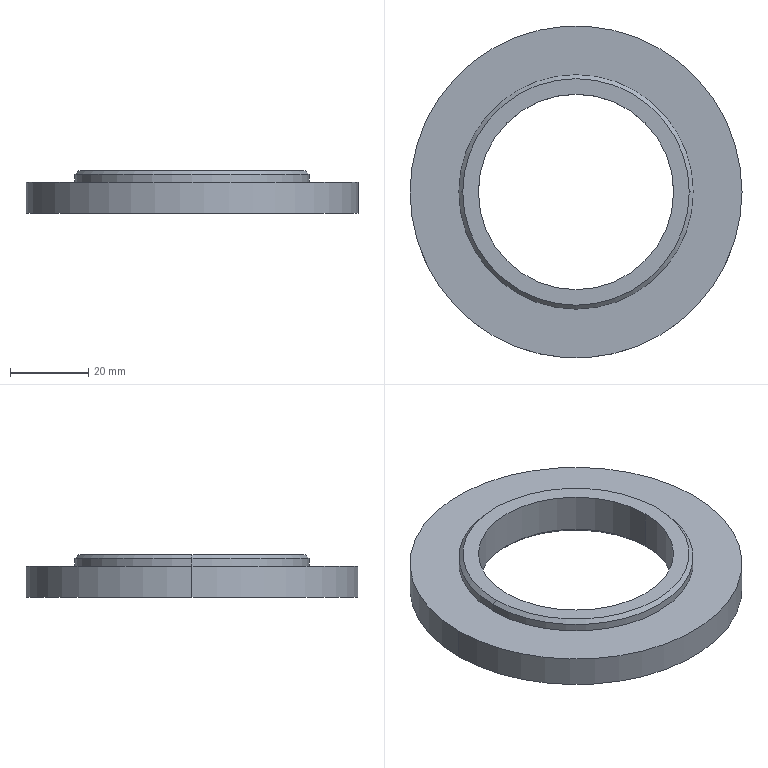Part | SolidWorks | features 3DProfileFeature 1, Chamfer 1, Extrusion 1, HoleWzd 1, ICE 1 | 1 solid | 37 faces | box 85 x 85 x 11 mm | volume 31782 mm3 | cylinder 18 | cone 16 | plane 3 | commonest cylinder face diameters 3.3 x12 50 x2 60 x2 85 x2
STEP:
#1=CARTESIAN_POINT('',(20.15,32.043,6.));
#2=VERTEX_POINT('',#1);
#3=CARTESIAN_POINT('',(16.85,32.043,6.));
#4=VERTEX_POINT('',#3);
#5=CARTESIAN_POINT('',(18.5,32.043,6.));
#6=DIRECTION('',(0.,0.,-1.));
#7=DIRECTION('',(-1.,0.,0.));
#8=AXIS2_PLACEMENT_3D('',#5,#6,#7);
#9=CIRCLE('',#8,1.65);
#10=EDGE_CURVE('',#2,#4,#9,.T.);
#11=ORIENTED_EDGE('',*,*,#10,.F.);
#12=CARTESIAN_POINT('',(20.15,32.043,0.));
#13=VERTEX_POINT('',#12);
#14=CARTESIAN_POINT('',(20.15,32.043,0.));
#15=DIRECTION('',(0.,0.,-1.));
#16=VECTOR('',#15,1000.);
#17=LINE('',#14,#16);
#18=EDGE_CURVE('',#2,#13,#17,.T.);
#19=ORIENTED_EDGE('',*,*,#18,.T.);
#20=CARTESIAN_POINT('',(16.85,32.043,0.));
#21=VERTEX_POINT('',#20);
#22=CARTESIAN_POINT('',(18.5,32.043,0.));
#23=DIRECTION('',(0.,0.,-1.));
#24=DIRECTION('',(-1.,0.,0.));
#25=AXIS2_PLACEMENT_3D('',#22,#23,#24);
#26=CIRCLE('',#25,1.65);
#27=EDGE_CURVE('',#13,#21,#26,.T.);
#28=ORIENTED_EDGE('',*,*,#27,.T.);
#29=CARTESIAN_POINT('',(16.85,32.043,0.));
#30=DIRECTION('',(0.,0.,-1.));
#31=VECTOR('',#30,1000.);
#32=LINE('',#29,#31);
#33=EDGE_CURVE('',#4,#21,#32,.T.);
#34=ORIENTED_EDGE('',*,*,#33,.F.);
#35=EDGE_LOOP('',(#11,#19,#28,#34));
#36=FACE_OUTER_BOUND('',#35,.T.);
#37=CARTESIAN_POINT('',(18.5,32.043,0.));
#38=DIRECTION('',(0.,0.,-1.));
#39=DIRECTION('',(-1.,0.,0.));
#40=AXIS2_PLACEMENT_3D('',#37,#38,#39);
#41=CYLINDRICAL_SURFACE('',#40,1.65);
#42=ADVANCED_FACE('',(#36),#41,.F.);
#43=CARTESIAN_POINT('',(18.5,32.043,6.991));
#44=VERTEX_POINT('',#43);
#45=CARTESIAN_POINT('',(16.85,32.043,6.));
#46=DIRECTION('',(-0.8572,0.,-0.515));
#47=VECTOR('',#46,1000.);
#48=LINE('',#45,#47);
#49=EDGE_CURVE('',#44,#4,#48,.T.);
#50=ORIENTED_EDGE('',*,*,#49,.F.);
#51=CARTESIAN_POINT('',(20.15,32.043,6.));
#52=DIRECTION('',(0.8572,0.,-0.515));
#53=VECTOR('',#52,1000.);
#54=LINE('',#51,#53);
#55=EDGE_CURVE('',#44,#2,#54,.T.);
#56=ORIENTED_EDGE('',*,*,#55,.T.);
#57=ORIENTED_EDGE('',*,*,#10,.T.);
#58=EDGE_LOOP('',(#50,#56,#57));
#59=FACE_OUTER_BOUND('',#58,.T.);
#60=CARTESIAN_POINT('',(18.5,32.043,6.));
#61=DIRECTION('',(0.,0.,-1.));
#62=DIRECTION('',(-1.,0.,0.));
#63=AXIS2_PLACEMENT_3D('',#60,#61,#62);
#64=CONICAL_SURFACE('',#63,1.65,1.03);
#65=ADVANCED_FACE('',(#59),#64,.F.);
#66=CARTESIAN_POINT('',(-16.85,32.043,6.));
#67=VERTEX_POINT('',#66);
#68=CARTESIAN_POINT('',(-20.15,32.043,6.));
#69=VERTEX_POINT('',#68);
#70=CARTESIAN_POINT('',(-18.5,32.043,6.));
#71=DIRECTION('',(0.,0.,-1.));
#72=DIRECTION('',(-1.,0.,0.));
#73=AXIS2_PLACEMENT_3D('',#70,#71,#72);
#74=CIRCLE('',#73,1.65);
#75=EDGE_CURVE('',#67,#69,#74,.T.);
#76=ORIENTED_EDGE('',*,*,#75,.F.);
#77=CARTESIAN_POINT('',(-16.85,32.043,0.));
#78=VERTEX_POINT('',#77);
#79=CARTESIAN_POINT('',(-16.85,32.043,0.));
#80=DIRECTION('',(0.,0.,-1.));
#81=VECTOR('',#80,1000.);
#82=LINE('',#79,#81);
#83=EDGE_CURVE('',#67,#78,#82,.T.);
#84=ORIENTED_EDGE('',*,*,#83,.T.);
#85=CARTESIAN_POINT('',(-20.15,32.043,0.));
#86=VERTEX_POINT('',#85);
#87=CARTESIAN_POINT('',(-18.5,32.043,0.));
#88=DIRECTION('',(0.,0.,-1.));
#89=DIRECTION('',(-1.,0.,0.));
#90=AXIS2_PLACEMENT_3D('',#87,#88,#89);
#91=CIRCLE('',#90,1.65);
#92=EDGE_CURVE('',#78,#86,#91,.T.);
#93=ORIENTED_EDGE('',*,*,#92,.T.);
#94=CARTESIAN_POINT('',(-20.15,32.043,0.));
#95=DIRECTION('',(0.,0.,-1.));
#96=VECTOR('',#95,1000.);
#97=LINE('',#94,#96);
#98=EDGE_CURVE('',#69,#86,#97,.T.);
#99=ORIENTED_EDGE('',*,*,#98,.F.);
#100=EDGE_LOOP('',(#76,#84,#93,#99));
#101=FACE_OUTER_BOUND('',#100,.T.);
#102=CARTESIAN_POINT('',(-18.5,32.043,0.));
#103=DIRECTION('',(0.,0.,-1.));
#104=DIRECTION('',(-1.,0.,0.));
#105=AXIS2_PLACEMENT_3D('',#102,#103,#104);
#106=CYLINDRICAL_SURFACE('',#105,1.65);
#107=ADVANCED_FACE('',(#101),#106,.F.);
#108=CARTESIAN_POINT('',(-18.5,32.043,6.991));
#109=VERTEX_POINT('',#108);
#110=CARTESIAN_POINT('',(-20.15,32.043,6.));
#111=DIRECTION('',(-0.8572,0.,-0.515));
#112=VECTOR('',#111,1000.);
#113=LINE('',#110,#112);
#114=EDGE_CURVE('',#109,#69,#113,.T.);
#115=ORIENTED_EDGE('',*,*,#114,.F.);
#116=CARTESIAN_POINT('',(-16.85,32.043,6.));
#117=DIRECTION('',(0.8572,0.,-0.515));
#118=VECTOR('',#117,1000.);
#119=LINE('',#116,#118);
#120=EDGE_CURVE('',#109,#67,#119,.T.);
#121=ORIENTED_EDGE('',*,*,#120,.T.);
#122=ORIENTED_EDGE('',*,*,#75,.T.);
#123=EDGE_LOOP('',(#115,#121,#122));
#124=FACE_OUTER_BOUND('',#123,.T.);
#125=CARTESIAN_POINT('',(-18.5,32.043,6.));
#126=DIRECTION('',(0.,0.,-1.));
#127=DIRECTION('',(-1.,0.,0.));
#128=AXIS2_PLACEMENT_3D('',#125,#126,#127);
#129=CONICAL_SURFACE('',#128,1.65,1.03);
#130=ADVANCED_FACE('',(#124),#129,.F.);
#131=CARTESIAN_POINT('',(-35.35,0.,6.));
#132=VERTEX_POINT('',#131);
#133=CARTESIAN_POINT('',(-38.65,0.,6.));
#134=VERTEX_POINT('',#133);
#135=CARTESIAN_POINT('',(-37.,0.,6.));
#136=DIRECTION('',(0.,0.,-1.));
#137=DIRECTION('',(-1.,0.,0.));
#138=AXIS2_PLACEMENT_3D('',#135,#136,#137);
#139=CIRCLE('',#138,1.65);
#140=EDGE_CURVE('',#132,#134,#139,.T.);
#141=ORIENTED_EDGE('',*,*,#140,.F.);
#142=CARTESIAN_POINT('',(-35.35,0.,0.));
#143=VERTEX_POINT('',#142);
#144=CARTESIAN_POINT('',(-35.35,0.,0.));
#145=DIRECTION('',(0.,0.,-1.));
#146=VECTOR('',#145,1000.);
#147=LINE('',#144,#146);
#148=EDGE_CURVE('',#132,#143,#147,.T.);
#149=ORIENTED_EDGE('',*,*,#148,.T.);
#150=CARTESIAN_POINT('',(-38.65,0.,0.));
#151=VERTEX_POINT('',#150);
#152=CARTESIAN_POINT('',(-37.,0.,0.));
#153=DIRECTION('',(0.,0.,-1.));
#154=DIRECTION('',(-1.,0.,0.));
#155=AXIS2_PLACEMENT_3D('',#152,#153,#154);
#156=CIRCLE('',#155,1.65);
#157=EDGE_CURVE('',#143,#151,#156,.T.);
#158=ORIENTED_EDGE('',*,*,#157,.T.);
#159=CARTESIAN_POINT('',(-38.65,0.,0.));
#160=DIRECTION('',(0.,0.,-1.));
#161=VECTOR('',#160,1000.);
#162=LINE('',#159,#161);
#163=EDGE_CURVE('',#134,#151,#162,.T.);
#164=ORIENTED_EDGE('',*,*,#163,.F.);
#165=EDGE_LOOP('',(#141,#149,#158,#164));
#166=FACE_OUTER_BOUND('',#165,.T.);
#167=CARTESIAN_POINT('',(-37.,0.,0.));
#168=DIRECTION('',(0.,0.,-1.));
#169=DIRECTION('',(-1.,0.,0.));
#170=AXIS2_PLACEMENT_3D('',#167,#168,#169);
#171=CYLINDRICAL_SURFACE('',#170,1.65);
#172=ADVANCED_FACE('',(#166),#171,.F.);
#173=CARTESIAN_POINT('',(-37.,0.,6.991));
#174=VERTEX_POINT('',#173);
#175=CARTESIAN_POINT('',(-38.65,0.,6.));
#176=DIRECTION('',(-0.8572,0.,-0.515));
#177=VECTOR('',#176,1000.);
#178=LINE('',#175,#177);
#179=EDGE_CURVE('',#174,#134,#178,.T.);
#180=ORIENTED_EDGE('',*,*,#179,.F.);
#181=CARTESIAN_POINT('',(-35.35,0.,6.));
#182=DIRECTION('',(0.8572,0.,-0.515));
#183=VECTOR('',#182,1000.);
#184=LINE('',#181,#183);
#185=EDGE_CURVE('',#174,#132,#184,.T.);
#186=ORIENTED_EDGE('',*,*,#185,.T.);
#187=ORIENTED_EDGE('',*,*,#140,.T.);
#188=EDGE_LOOP('',(#180,#186,#187));
#189=FACE_OUTER_BOUND('',#188,.T.);
#190=CARTESIAN_POINT('',(-37.,0.,6.));
#191=DIRECTION('',(0.,0.,-1.));
#192=DIRECTION('',(-1.,0.,0.));
#193=AXIS2_PLACEMENT_3D('',#190,#191,#192);
#194=CONICAL_SURFACE('',#193,1.65,1.03);
#195=ADVANCED_FACE('',(#189),#194,.F.);
#196=CARTESIAN_POINT('',(-16.85,-32.043,6.));
#197=VERTEX_POINT('',#196);
#198=CARTESIAN_POINT('',(-20.15,-32.043,6.));
#199=VERTEX_POINT('',#198);
#200=CARTESIAN_POINT('',(-18.5,-32.043,6.));
#201=DIRECTION('',(0.,0.,-1.));
#202=DIRECTION('',(-1.,0.,0.));
#203=AXIS2_PLACEMENT_3D('',#200,#201,#202);
#204=CIRCLE('',#203,1.65);
#205=EDGE_CURVE('',#197,#199,#204,.T.);
#206=ORIENTED_EDGE('',*,*,#205,.F.);
#207=CARTESIAN_POINT('',(-16.85,-32.043,0.));
#208=VERTEX_POINT('',#207);
#209=CARTESIAN_POINT('',(-16.85,-32.043,0.));
#210=DIRECTION('',(0.,0.,-1.));
#211=VECTOR('',#210,1000.);
#212=LINE('',#209,#211);
#213=EDGE_CURVE('',#197,#208,#212,.T.);
#214=ORIENTED_EDGE('',*,*,#213,.T.);
#215=CARTESIAN_POINT('',(-20.15,-32.043,0.));
#216=VERTEX_POINT('',#215);
#217=CARTESIAN_POINT('',(-18.5,-32.043,0.));
#218=DIRECTION('',(0.,0.,-1.));
#219=DIRECTION('',(-1.,0.,0.));
#220=AXIS2_PLACEMENT_3D('',#217,#218,#219);
#221=CIRCLE('',#220,1.65);
#222=EDGE_CURVE('',#208,#216,#221,.T.);
#223=ORIENTED_EDGE('',*,*,#222,.T.);
#224=CARTESIAN_POINT('',(-20.15,-32.043,0.));
#225=DIRECTION('',(0.,0.,-1.));
#226=VECTOR('',#225,1000.);
#227=LINE('',#224,#226);
#228=EDGE_CURVE('',#199,#216,#227,.T.);
#229=ORIENTED_EDGE('',*,*,#228,.F.);
#230=EDGE_LOOP('',(#206,#214,#223,#229));
#231=FACE_OUTER_BOUND('',#230,.T.);
#232=CARTESIAN_POINT('',(-18.5,-32.043,0.));
#233=DIRECTION('',(0.,0.,-1.));
#234=DIRECTION('',(-1.,0.,0.));
#235=AXIS2_PLACEMENT_3D('',#232,#233,#234);
#236=CYLINDRICAL_SURFACE('',#235,1.65);
#237=ADVANCED_FACE('',(#231),#236,.F.);
#238=CARTESIAN_POINT('',(-18.5,-32.043,6.991));
#239=VERTEX_POINT('',#238);
#240=CARTESIAN_POINT('',(-20.15,-32.043,6.));
#241=DIRECTION('',(-0.8572,0.,-0.515));
#242=VECTOR('',#241,1000.);
#243=LINE('',#240,#242);
#244=EDGE_CURVE('',#239,#199,#243,.T.);
#245=ORIENTED_EDGE('',*,*,#244,.F.);
#246=CARTESIAN_POINT('',(-16.85,-32.043,6.));
#247=DIRECTION('',(0.8572,0.,-0.515));
#248=VECTOR('',#247,1000.);
#249=LINE('',#246,#248);
#250=EDGE_CURVE('',#239,#197,#249,.T.);
#251=ORIENTED_EDGE('',*,*,#250,.T.);
#252=ORIENTED_EDGE('',*,*,#205,.T.);
#253=EDGE_LOOP('',(#245,#251,#252));
#254=FACE_OUTER_BOUND('',#253,.T.);
#255=CARTESIAN_POINT('',(-18.5,-32.043,6.));
#256=DIRECTION('',(0.,0.,-1.));
#257=DIRECTION('',(-1.,0.,0.));
#258=AXIS2_PLACEMENT_3D('',#255,#256,#257);
#259=CONICAL_SURFACE('',#258,1.65,1.03);
#260=ADVANCED_FACE('',(#254),#259,.F.);
#261=CARTESIAN_POINT('',(20.15,-32.043,6.));
#262=VERTEX_POINT('',#261);
#263=CARTESIAN_POINT('',(16.85,-32.043,6.));
#264=VERTEX_POINT('',#263);
#265=CARTESIAN_POINT('',(18.5,-32.043,6.));
#266=DIRECTION('',(0.,0.,-1.));
#267=DIRECTION('',(-1.,0.,0.));
#268=AXIS2_PLACEMENT_3D('',#265,#266,#267);
#269=CIRCLE('',#268,1.65);
#270=EDGE_CURVE('',#262,#264,#269,.T.);
#271=ORIENTED_EDGE('',*,*,#270,.F.);
#272=CARTESIAN_POINT('',(20.15,-32.043,0.));
#273=VERTEX_POINT('',#272);
#274=CARTESIAN_POINT('',(20.15,-32.043,0.));
#275=DIRECTION('',(0.,0.,-1.));
#276=VECTOR('',#275,1000.);
#277=LINE('',#274,#276);
#278=EDGE_CURVE('',#262,#273,#277,.T.);
#279=ORIENTED_EDGE('',*,*,#278,.T.);
#280=CARTESIAN_POINT('',(16.85,-32.043,0.));
#281=VERTEX_POINT('',#280);
#282=CARTESIAN_POINT('',(18.5,-32.043,0.));
#283=DIRECTION('',(0.,0.,-1.));
#284=DIRECTION('',(-1.,0.,0.));
#285=AXIS2_PLACEMENT_3D('',#282,#283,#284);
#286=CIRCLE('',#285,1.65);
#287=EDGE_CURVE('',#273,#281,#286,.T.);
#288=ORIENTED_EDGE('',*,*,#287,.T.);
#289=CARTESIAN_POINT('',(16.85,-32.043,0.));
#290=DIRECTION('',(0.,0.,-1.));
#291=VECTOR('',#290,1000.);
#292=LINE('',#289,#291);
#293=EDGE_CURVE('',#264,#281,#292,.T.);
#294=ORIENTED_EDGE('',*,*,#293,.F.);
#295=EDGE_LOOP('',(#271,#279,#288,#294));
#296=FACE_OUTER_BOUND('',#295,.T.);
#297=CARTESIAN_POINT('',(18.5,-32.043,0.));
#298=DIRECTION('',(0.,0.,-1.));
#299=DIRECTION('',(-1.,0.,0.));
#300=AXIS2_PLACEMENT_3D('',#297,#298,#299);
#301=CYLINDRICAL_SURFACE('',#300,1.65);
#302=ADVANCED_FACE('',(#296),#301,.F.);
#303=CARTESIAN_POINT('',(18.5,-32.043,6.991));
#304=VERTEX_POINT('',#303);
#305=CARTESIAN_POINT('',(16.85,-32.043,6.));
#306=DIRECTION('',(-0.8572,0.,-0.515));
#307=VECTOR('',#306,1000.);
#308=LINE('',#305,#307);
#309=EDGE_CURVE('',#304,#264,#308,.T.);
#310=ORIENTED_EDGE('',*,*,#309,.F.);
#311=CARTESIAN_POINT('',(20.15,-32.043,6.));
#312=DIRECTION('',(0.8572,0.,-0.515));
#313=VECTOR('',#312,1000.);
#314=LINE('',#311,#313);
#315=EDGE_CURVE('',#304,#262,#314,.T.);
#316=ORIENTED_EDGE('',*,*,#315,.T.);
#317=ORIENTED_EDGE('',*,*,#270,.T.);
#318=EDGE_LOOP('',(#310,#316,#317));
#319=FACE_OUTER_BOUND('',#318,.T.);
#320=CARTESIAN_POINT('',(18.5,-32.043,6.));
#321=DIRECTION('',(0.,0.,-1.));
#322=DIRECTION('',(-1.,0.,0.));
#323=AXIS2_PLACEMENT_3D('',#320,#321,#322);
#324=CONICAL_SURFACE('',#323,1.65,1.03);
#325=ADVANCED_FACE('',(#319),#324,.F.);
#326=CARTESIAN_POINT('',(38.65,0.,6.));
#327=VERTEX_POINT('',#326);
#328=CARTESIAN_POINT('',(35.35,0.,6.));
#329=VERTEX_POINT('',#328);
#330=CARTESIAN_POINT('',(37.,0.,6.));
#331=DIRECTION('',(0.,0.,-1.));
#332=DIRECTION('',(-1.,0.,0.));
#333=AXIS2_PLACEMENT_3D('',#330,#331,#332);
#334=CIRCLE('',#333,1.65);
#335=EDGE_CURVE('',#327,#329,#334,.T.);
#336=ORIENTED_EDGE('',*,*,#335,.F.);
#337=CARTESIAN_POINT('',(38.65,0.,0.));
#338=VERTEX_POINT('',#337);
#339=CARTESIAN_POINT('',(38.65,0.,0.));
#340=DIRECTION('',(0.,0.,-1.));
#341=VECTOR('',#340,1000.);
#342=LINE('',#339,#341);
#343=EDGE_CURVE('',#327,#338,#342,.T.);
#344=ORIENTED_EDGE('',*,*,#343,.T.);
#345=CARTESIAN_POINT('',(35.35,0.,0.));
#346=VERTEX_POINT('',#345);
#347=CARTESIAN_POINT('',(37.,0.,0.));
#348=DIRECTION('',(0.,0.,-1.));
#349=DIRECTION('',(-1.,0.,0.));
#350=AXIS2_PLACEMENT_3D('',#347,#348,#349);
#351=CIRCLE('',#350,1.65);
#352=EDGE_CURVE('',#338,#346,#351,.T.);
#353=ORIENTED_EDGE('',*,*,#352,.T.);
#354=CARTESIAN_POINT('',(35.35,0.,0.));
#355=DIRECTION('',(0.,0.,-1.));
#356=VECTOR('',#355,1000.);
#357=LINE('',#354,#356);
#358=EDGE_CURVE('',#329,#346,#357,.T.);
#359=ORIENTED_EDGE('',*,*,#358,.F.);
#360=EDGE_LOOP('',(#336,#344,#353,#359));
#361=FACE_OUTER_BOUND('',#360,.T.);
#362=CARTESIAN_POINT('',(37.,0.,0.));
#363=DIRECTION('',(0.,0.,-1.));
#364=DIRECTION('',(-1.,0.,0.));
#365=AXIS2_PLACEMENT_3D('',#362,#363,#364);
#366=CYLINDRICAL_SURFACE('',#365,1.65);
#367=ADVANCED_FACE('',(#361),#366,.F.);
#368=CARTESIAN_POINT('',(37.,0.,6.991));
#369=VERTEX_POINT('',#368);
#370=CARTESIAN_POINT('',(35.35,0.,6.));
#371=DIRECTION('',(-0.8572,0.,-0.515));
#372=VECTOR('',#371,1000.);
#373=LINE('',#370,#372);
#374=EDGE_CURVE('',#369,#329,#373,.T.);
#375=ORIENTED_EDGE('',*,*,#374,.F.);
#376=CARTESIAN_POINT('',(38.65,0.,6.));
#377=DIRECTION('',(0.8572,0.,-0.515));
#378=VECTOR('',#377,1000.);
#379=LINE('',#376,#378);
#380=EDGE_CURVE('',#369,#327,#379,.T.);
#381=ORIENTED_EDGE('',*,*,#380,.T.);
#382=ORIENTED_EDGE('',*,*,#335,.T.);
#383=EDGE_LOOP('',(#375,#381,#382));
#384=FACE_OUTER_BOUND('',#383,.T.);
#385=CARTESIAN_POINT('',(37.,0.,6.));
#386=DIRECTION('',(0.,0.,-1.));
#387=DIRECTION('',(-1.,0.,0.));
#388=AXIS2_PLACEMENT_3D('',#385,#386,#387);
#389=CONICAL_SURFACE('',#388,1.65,1.03);
#390=ADVANCED_FACE('',(#384),#389,.F.);
#391=CARTESIAN_POINT('',(25.,0.,1.));
#392=VERTEX_POINT('',#391);
#393=CARTESIAN_POINT('',(-25.,0.,1.));
#394=VERTEX_POINT('',#393);
#395=CARTESIAN_POINT('',(0.,0.,1.));
#396=DIRECTION('',(0.,0.,-1.));
#397=DIRECTION('',(1.,0.,0.));
#398=AXIS2_PLACEMENT_3D('',#395,#396,#397);
#399=CIRCLE('',#398,25.);
#400=EDGE_CURVE('',#392,#394,#399,.T.);
#401=ORIENTED_EDGE('',*,*,#400,.F.);
#402=CARTESIAN_POINT('',(26.,0.,0.));
#403=VERTEX_POINT('',#402);
#404=CARTESIAN_POINT('',(26.,0.,0.));
#405=DIRECTION('',(0.7071,0.,-0.7071));
#406=VECTOR('',#405,1000.);
#407=LINE('',#404,#406);
#408=EDGE_CURVE('',#392,#403,#407,.T.);
#409=ORIENTED_EDGE('',*,*,#408,.T.);
#410=CARTESIAN_POINT('',(-26.,0.,0.));
#411=VERTEX_POINT('',#410);
#412=CARTESIAN_POINT('',(0.,0.,0.));
#413=DIRECTION('',(0.,0.,1.));
#414=DIRECTION('',(1.,0.,0.));
#415=AXIS2_PLACEMENT_3D('',#412,#413,#414);
#416=CIRCLE('',#415,26.);
#417=EDGE_CURVE('',#411,#403,#416,.T.);
#418=ORIENTED_EDGE('',*,*,#417,.F.);
#419=CARTESIAN_POINT('',(-26.,0.,0.));
#420=DIRECTION('',(-0.7071,0.,-0.7071));
#421=VECTOR('',#420,1000.);
#422=LINE('',#419,#421);
#423=EDGE_CURVE('',#394,#411,#422,.T.);
#424=ORIENTED_EDGE('',*,*,#423,.F.);
#425=EDGE_LOOP('',(#401,#409,#418,#424));
#426=FACE_OUTER_BOUND('',#425,.T.);
#427=CARTESIAN_POINT('',(0.,0.,0.));
#428=DIRECTION('',(0.,0.,-1.));
#429=DIRECTION('',(-1.,0.,0.));
#430=AXIS2_PLACEMENT_3D('',#427,#428,#429);
#431=CONICAL_SURFACE('',#430,26.,0.7854);
#432=ADVANCED_FACE('',(#426),#431,.F.);
#433=CARTESIAN_POINT('',(29.,0.,11.));
#434=VERTEX_POINT('',#433);
#435=CARTESIAN_POINT('',(-29.,0.,11.));
#436=VERTEX_POINT('',#435);
#437=CARTESIAN_POINT('',(0.,0.,11.));
#438=DIRECTION('',(0.,0.,1.));
#439=DIRECTION('',(1.,0.,0.));
#440=AXIS2_PLACEMENT_3D('',#437,#438,#439);
#441=CIRCLE('',#440,29.);
#442=EDGE_CURVE('',#434,#436,#441,.T.);
#443=ORIENTED_EDGE('',*,*,#442,.F.);
#444=CARTESIAN_POINT('',(30.,0.,10.));
#445=VERTEX_POINT('',#444);
#446=CARTESIAN_POINT('',(29.,0.,11.));
#447=DIRECTION('',(0.7071,0.,-0.7071));
#448=VECTOR('',#447,1000.);
#449=LINE('',#446,#448);
#450=EDGE_CURVE('',#434,#445,#449,.T.);
#451=ORIENTED_EDGE('',*,*,#450,.T.);
#452=CARTESIAN_POINT('',(-30.,0.,10.));
#453=VERTEX_POINT('',#452);
#454=CARTESIAN_POINT('',(0.,0.,10.));
#455=DIRECTION('',(0.,0.,-1.));
#456=DIRECTION('',(1.,0.,0.));
#457=AXIS2_PLACEMENT_3D('',#454,#455,#456);
#458=CIRCLE('',#457,30.);
#459=EDGE_CURVE('',#453,#445,#458,.T.);
#460=ORIENTED_EDGE('',*,*,#459,.F.);
#461=CARTESIAN_POINT('',(-29.,0.,11.));
#462=DIRECTION('',(-0.7071,0.,-0.7071));
#463=VECTOR('',#462,1000.);
#464=LINE('',#461,#463);
#465=EDGE_CURVE('',#436,#453,#464,.T.);
#466=ORIENTED_EDGE('',*,*,#465,.F.);
#467=EDGE_LOOP('',(#443,#451,#460,#466));
#468=FACE_OUTER_BOUND('',#467,.T.);
#469=CARTESIAN_POINT('',(0.,0.,11.));
#470=DIRECTION('',(0.,0.,-1.));
#471=DIRECTION('',(-1.,0.,0.));
#472=AXIS2_PLACEMENT_3D('',#469,#470,#471);
#473=CONICAL_SURFACE('',#472,29.,0.7854);
#474=ADVANCED_FACE('',(#468),#473,.T.);
#475=ORIENTED_EDGE('',*,*,#459,.T.);
#476=CARTESIAN_POINT('',(30.,0.,8.));
#477=VERTEX_POINT('',#476);
#478=CARTESIAN_POINT('',(30.,0.,11.));
#479=DIRECTION('',(0.,0.,-1.));
#480=VECTOR('',#479,1000.);
#481=LINE('',#478,#480);
#482=EDGE_CURVE('',#445,#477,#481,.T.);
#483=ORIENTED_EDGE('',*,*,#482,.T.);
#484=CARTESIAN_POINT('',(-30.,0.,8.));
#485=VERTEX_POINT('',#484);
#486=CARTESIAN_POINT('',(0.,0.,8.));
#487=DIRECTION('',(0.,0.,1.));
#488=DIRECTION('',(1.,0.,0.));
#489=AXIS2_PLACEMENT_3D('',#486,#487,#488);
#490=CIRCLE('',#489,30.);
#491=EDGE_CURVE('',#477,#485,#490,.T.);
#492=ORIENTED_EDGE('',*,*,#491,.T.);
#493=CARTESIAN_POINT('',(-30.,0.,11.));
#494=DIRECTION('',(0.,0.,-1.));
#495=VECTOR('',#494,1000.);
#496=LINE('',#493,#495);
#497=EDGE_CURVE('',#453,#485,#496,.T.);
#498=ORIENTED_EDGE('',*,*,#497,.F.);
#499=EDGE_LOOP('',(#475,#483,#492,#498));
#500=FACE_OUTER_BOUND('',#499,.T.);
#501=CARTESIAN_POINT('',(0.,0.,11.));
#502=DIRECTION('',(0.,0.,-1.));
#503=DIRECTION('',(-1.,0.,0.));
#504=AXIS2_PLACEMENT_3D('',#501,#502,#503);
#505=CYLINDRICAL_SURFACE('',#504,30.);
#506=ADVANCED_FACE('',(#500),#505,.T.);
#507=CARTESIAN_POINT('',(-25.,0.,11.));
#508=VERTEX_POINT('',#507);
#509=CARTESIAN_POINT('',(25.,0.,11.));
#510=VERTEX_POINT('',#509);
#511=CARTESIAN_POINT('',(0.,0.,11.));
#512=DIRECTION('',(0.,0.,1.));
#513=DIRECTION('',(1.,0.,0.));
#514=AXIS2_PLACEMENT_3D('',#511,#512,#513);
#515=CIRCLE('',#514,25.);
#516=EDGE_CURVE('',#508,#510,#515,.T.);
#517=ORIENTED_EDGE('',*,*,#516,.T.);
#518=CARTESIAN_POINT('',(25.,0.,8.));
#519=DIRECTION('',(0.,0.,-1.));
#520=VECTOR('',#519,1000.);
#521=LINE('',#518,#520);
#522=EDGE_CURVE('',#510,#392,#521,.T.);
#523=ORIENTED_EDGE('',*,*,#522,.T.);
#524=ORIENTED_EDGE('',*,*,#400,.T.);
#525=CARTESIAN_POINT('',(-25.,0.,8.));
#526=DIRECTION('',(0.,0.,-1.));
#527=VECTOR('',#526,1000.);
#528=LINE('',#525,#527);
#529=EDGE_CURVE('',#508,#394,#528,.T.);
#530=ORIENTED_EDGE('',*,*,#529,.F.);
#531=EDGE_LOOP('',(#517,#523,#524,#530));
#532=FACE_OUTER_BOUND('',#531,.T.);
#533=CARTESIAN_POINT('',(0.,0.,8.));
#534=DIRECTION('',(0.,0.,-1.));
#535=DIRECTION('',(-1.,0.,0.));
#536=AXIS2_PLACEMENT_3D('',#533,#534,#535);
#537=CYLINDRICAL_SURFACE('',#536,25.);
#538=ADVANCED_FACE('',(#532),#537,.F.);
#539=CARTESIAN_POINT('',(42.5,0.,8.));
#540=VERTEX_POINT('',#539);
#541=CARTESIAN_POINT('',(-42.5,0.,8.));
#542=VERTEX_POINT('',#541);
#543=CARTESIAN_POINT('',(0.,0.,8.));
#544=DIRECTION('',(0.,0.,1.));
#545=DIRECTION('',(1.,0.,0.));
#546=AXIS2_PLACEMENT_3D('',#543,#544,#545);
#547=CIRCLE('',#546,42.5);
#548=EDGE_CURVE('',#540,#542,#547,.T.);
#549=ORIENTED_EDGE('',*,*,#548,.F.);
#550=CARTESIAN_POINT('',(42.5,0.,0.));
#551=VERTEX_POINT('',#550);
#552=CARTESIAN_POINT('',(42.5,0.,8.));
#553=DIRECTION('',(0.,0.,-1.));
#554=VECTOR('',#553,1000.);
#555=LINE('',#552,#554);
#556=EDGE_CURVE('',#540,#551,#555,.T.);
#557=ORIENTED_EDGE('',*,*,#556,.T.);
#558=CARTESIAN_POINT('',(-42.5,0.,0.));
#559=VERTEX_POINT('',#558);
#560=CARTESIAN_POINT('',(0.,0.,0.));
#561=DIRECTION('',(0.,0.,1.));
#562=DIRECTION('',(1.,0.,0.));
#563=AXIS2_PLACEMENT_3D('',#560,#561,#562);
#564=CIRCLE('',#563,42.5);
#565=EDGE_CURVE('',#551,#559,#564,.T.);
#566=ORIENTED_EDGE('',*,*,#565,.T.);
#567=CARTESIAN_POINT('',(-42.5,0.,8.));
#568=DIRECTION('',(0.,0.,-1.));
#569=VECTOR('',#568,1000.);
#570=LINE('',#567,#569);
#571=EDGE_CURVE('',#542,#559,#570,.T.);
#572=ORIENTED_EDGE('',*,*,#571,.F.);
#573=EDGE_LOOP('',(#549,#557,#566,#572));
#574=FACE_OUTER_BOUND('',#573,.T.);
#575=CARTESIAN_POINT('',(0.,0.,8.));
#576=DIRECTION('',(0.,0.,-1.));
#577=DIRECTION('',(-1.,0.,0.));
#578=AXIS2_PLACEMENT_3D('',#575,#576,#577);
#579=CYLINDRICAL_SURFACE('',#578,42.5);
#580=ADVANCED_FACE('',(#574),#579,.T.);
#581=CARTESIAN_POINT('',(0.,0.,8.));
#582=DIRECTION('',(0.,0.,1.));
#583=DIRECTION('',(1.,0.,0.));
#584=AXIS2_PLACEMENT_3D('',#581,#582,#583);
#585=CIRCLE('',#584,42.5);
#586=EDGE_CURVE('',#542,#540,#585,.T.);
#587=ORIENTED_EDGE('',*,*,#586,.T.);
#588=ORIENTED_EDGE('',*,*,#548,.T.);
#589=EDGE_LOOP('',(#587,#588));
#590=FACE_OUTER_BOUND('',#589,.T.);
#591=CARTESIAN_POINT('',(0.,0.,8.));
#592=DIRECTION('',(0.,0.,1.));
#593=DIRECTION('',(1.,0.,0.));
#594=AXIS2_PLACEMENT_3D('',#591,#592,#593);
#595=CIRCLE('',#594,30.);
#596=EDGE_CURVE('',#485,#477,#595,.T.);
#597=ORIENTED_EDGE('',*,*,#596,.F.);
#598=ORIENTED_EDGE('',*,*,#491,.F.);
#599=EDGE_LOOP('',(#597,#598));
#600=FACE_BOUND('',#599,.T.);
#601=CARTESIAN_POINT('',(0.,0.,8.));
#602=DIRECTION('',(0.,0.,1.));
#603=DIRECTION('',(1.,0.,0.));
#604=AXIS2_PLACEMENT_3D('',#601,#602,#603);
#605=PLANE('',#604);
#606=ADVANCED_FACE('',(#590,#600),#605,.T.);
#607=CARTESIAN_POINT('',(18.5,32.043,0.));
#608=DIRECTION('',(0.,0.,-1.));
#609=DIRECTION('',(-1.,0.,0.));
#610=AXIS2_PLACEMENT_3D('',#607,#608,#609);
#611=CIRCLE('',#610,1.65);
#612=EDGE_CURVE('',#21,#13,#611,.T.);
#613=ORIENTED_EDGE('',*,*,#612,.F.);
#614=ORIENTED_EDGE('',*,*,#27,.F.);
#615=EDGE_LOOP('',(#613,#614));
#616=FACE_BOUND('',#615,.T.);
#617=CARTESIAN_POINT('',(-18.5,32.043,0.));
#618=DIRECTION('',(0.,0.,-1.));
#619=DIRECTION('',(-1.,0.,0.));
#620=AXIS2_PLACEMENT_3D('',#617,#618,#619);
#621=CIRCLE('',#620,1.65);
#622=EDGE_CURVE('',#86,#78,#621,.T.);
#623=ORIENTED_EDGE('',*,*,#622,.F.);
#624=ORIENTED_EDGE('',*,*,#92,.F.);
#625=EDGE_LOOP('',(#623,#624));
#626=FACE_BOUND('',#625,.T.);
#627=CARTESIAN_POINT('',(-37.,0.,0.));
#628=DIRECTION('',(0.,0.,-1.));
#629=DIRECTION('',(-1.,0.,0.));
#630=AXIS2_PLACEMENT_3D('',#627,#628,#629);
#631=CIRCLE('',#630,1.65);
#632=EDGE_CURVE('',#151,#143,#631,.T.);
#633=ORIENTED_EDGE('',*,*,#632,.F.);
#634=ORIENTED_EDGE('',*,*,#157,.F.);
#635=EDGE_LOOP('',(#633,#634));
#636=FACE_BOUND('',#635,.T.);
#637=CARTESIAN_POINT('',(-18.5,-32.043,0.));
#638=DIRECTION('',(0.,0.,-1.));
#639=DIRECTION('',(-1.,0.,0.));
#640=AXIS2_PLACEMENT_3D('',#637,#638,#639);
#641=CIRCLE('',#640,1.65);
#642=EDGE_CURVE('',#216,#208,#641,.T.);
#643=ORIENTED_EDGE('',*,*,#642,.F.);
#644=ORIENTED_EDGE('',*,*,#222,.F.);
#645=EDGE_LOOP('',(#643,#644));
#646=FACE_BOUND('',#645,.T.);
#647=CARTESIAN_POINT('',(18.5,-32.043,0.));
#648=DIRECTION('',(0.,0.,-1.));
#649=DIRECTION('',(-1.,0.,0.));
#650=AXIS2_PLACEMENT_3D('',#647,#648,#649);
#651=CIRCLE('',#650,1.65);
#652=EDGE_CURVE('',#281,#273,#651,.T.);
#653=ORIENTED_EDGE('',*,*,#652,.F.);
#654=ORIENTED_EDGE('',*,*,#287,.F.);
#655=EDGE_LOOP('',(#653,#654));
#656=FACE_BOUND('',#655,.T.);
#657=CARTESIAN_POINT('',(37.,0.,0.));
#658=DIRECTION('',(0.,0.,-1.));
#659=DIRECTION('',(-1.,0.,0.));
#660=AXIS2_PLACEMENT_3D('',#657,#658,#659);
#661=CIRCLE('',#660,1.65);
#662=EDGE_CURVE('',#346,#338,#661,.T.);
#663=ORIENTED_EDGE('',*,*,#662,.F.);
#664=ORIENTED_EDGE('',*,*,#352,.F.);
#665=EDGE_LOOP('',(#663,#664));
#666=FACE_BOUND('',#665,.T.);
#667=ORIENTED_EDGE('',*,*,#417,.T.);
#668=CARTESIAN_POINT('',(0.,0.,0.));
#669=DIRECTION('',(0.,0.,1.));
#670=DIRECTION('',(1.,0.,0.));
#671=AXIS2_PLACEMENT_3D('',#668,#669,#670);
#672=CIRCLE('',#671,26.);
#673=EDGE_CURVE('',#403,#411,#672,.T.);
#674=ORIENTED_EDGE('',*,*,#673,.T.);
#675=EDGE_LOOP('',(#667,#674));
#676=FACE_BOUND('',#675,.T.);
#677=CARTESIAN_POINT('',(0.,0.,0.));
#678=DIRECTION('',(0.,0.,1.));
#679=DIRECTION('',(1.,0.,0.));
#680=AXIS2_PLACEMENT_3D('',#677,#678,#679);
#681=CIRCLE('',#680,42.5);
#682=EDGE_CURVE('',#559,#551,#681,.T.);
#683=ORIENTED_EDGE('',*,*,#682,.F.);
#684=ORIENTED_EDGE('',*,*,#565,.F.);
#685=EDGE_LOOP('',(#683,#684));
#686=FACE_OUTER_BOUND('',#685,.T.);
#687=CARTESIAN_POINT('',(0.,0.,0.));
#688=DIRECTION('',(0.,0.,1.));
#689=DIRECTION('',(1.,0.,0.));
#690=AXIS2_PLACEMENT_3D('',#687,#688,#689);
#691=PLANE('',#690);
#692=ADVANCED_FACE('',(#616,#626,#636,#646,#656,#666,#676,#686),#691,.F.);
#693=ORIENTED_EDGE('',*,*,#556,.F.);
#694=ORIENTED_EDGE('',*,*,#586,.F.);
#695=ORIENTED_EDGE('',*,*,#571,.T.);
#696=ORIENTED_EDGE('',*,*,#682,.T.);
#697=EDGE_LOOP('',(#693,#694,#695,#696));
#698=FACE_OUTER_BOUND('',#697,.T.);
#699=CARTESIAN_POINT('',(0.,0.,8.));
#700=DIRECTION('',(0.,0.,-1.));
#701=DIRECTION('',(-1.,0.,0.));
#702=AXIS2_PLACEMENT_3D('',#699,#700,#701);
#703=CYLINDRICAL_SURFACE('',#702,42.5);
#704=ADVANCED_FACE('',(#698),#703,.T.);
#705=ORIENTED_EDGE('',*,*,#522,.F.);
#706=CARTESIAN_POINT('',(0.,0.,11.));
#707=DIRECTION('',(0.,0.,1.));
#708=DIRECTION('',(1.,0.,0.));
#709=AXIS2_PLACEMENT_3D('',#706,#707,#708);
#710=CIRCLE('',#709,25.);
#711=EDGE_CURVE('',#510,#508,#710,.T.);
#712=ORIENTED_EDGE('',*,*,#711,.T.);
#713=ORIENTED_EDGE('',*,*,#529,.T.);
#714=CARTESIAN_POINT('',(0.,0.,1.));
#715=DIRECTION('',(0.,0.,-1.));
#716=DIRECTION('',(1.,0.,0.));
#717=AXIS2_PLACEMENT_3D('',#714,#715,#716);
#718=CIRCLE('',#717,25.);
#719=EDGE_CURVE('',#394,#392,#718,.T.);
#720=ORIENTED_EDGE('',*,*,#719,.T.);
#721=EDGE_LOOP('',(#705,#712,#713,#720));
#722=FACE_OUTER_BOUND('',#721,.T.);
#723=CARTESIAN_POINT('',(0.,0.,8.));
#724=DIRECTION('',(0.,0.,-1.));
#725=DIRECTION('',(-1.,0.,0.));
#726=AXIS2_PLACEMENT_3D('',#723,#724,#725);
#727=CYLINDRICAL_SURFACE('',#726,25.);
#728=ADVANCED_FACE('',(#722),#727,.F.);
#729=CARTESIAN_POINT('',(0.,0.,11.));
#730=DIRECTION('',(0.,0.,1.));
#731=DIRECTION('',(1.,0.,0.));
#732=AXIS2_PLACEMENT_3D('',#729,#730,#731);
#733=CIRCLE('',#732,29.);
#734=EDGE_CURVE('',#436,#434,#733,.T.);
#735=ORIENTED_EDGE('',*,*,#734,.T.);
#736=ORIENTED_EDGE('',*,*,#442,.T.);
#737=EDGE_LOOP('',(#735,#736));
#738=FACE_OUTER_BOUND('',#737,.T.);
#739=ORIENTED_EDGE('',*,*,#516,.F.);
#740=ORIENTED_EDGE('',*,*,#711,.F.);
#741=EDGE_LOOP('',(#739,#740));
#742=FACE_BOUND('',#741,.T.);
#743=CARTESIAN_POINT('',(0.,0.,11.));
#744=DIRECTION('',(0.,0.,1.));
#745=DIRECTION('',(1.,0.,0.));
#746=AXIS2_PLACEMENT_3D('',#743,#744,#745);
#747=PLANE('',#746);
#748=ADVANCED_FACE('',(#738,#742),#747,.T.);
#749=ORIENTED_EDGE('',*,*,#482,.F.);
#750=CARTESIAN_POINT('',(0.,0.,10.));
#751=DIRECTION('',(0.,0.,-1.));
#752=DIRECTION('',(1.,0.,0.));
#753=AXIS2_PLACEMENT_3D('',#750,#751,#752);
#754=CIRCLE('',#753,30.);
#755=EDGE_CURVE('',#445,#453,#754,.T.);
#756=ORIENTED_EDGE('',*,*,#755,.T.);
#757=ORIENTED_EDGE('',*,*,#497,.T.);
#758=ORIENTED_EDGE('',*,*,#596,.T.);
#759=EDGE_LOOP('',(#749,#756,#757,#758));
#760=FACE_OUTER_BOUND('',#759,.T.);
#761=CARTESIAN_POINT('',(0.,0.,11.));
#762=DIRECTION('',(0.,0.,-1.));
#763=DIRECTION('',(-1.,0.,0.));
#764=AXIS2_PLACEMENT_3D('',#761,#762,#763);
#765=CYLINDRICAL_SURFACE('',#764,30.);
#766=ADVANCED_FACE('',(#760),#765,.T.);
#767=ORIENTED_EDGE('',*,*,#450,.F.);
#768=ORIENTED_EDGE('',*,*,#734,.F.);
#769=ORIENTED_EDGE('',*,*,#465,.T.);
#770=ORIENTED_EDGE('',*,*,#755,.F.);
#771=EDGE_LOOP('',(#767,#768,#769,#770));
#772=FACE_OUTER_BOUND('',#771,.T.);
#773=CARTESIAN_POINT('',(0.,0.,11.));
#774=DIRECTION('',(0.,0.,-1.));
#775=DIRECTION('',(-1.,0.,0.));
#776=AXIS2_PLACEMENT_3D('',#773,#774,#775);
#777=CONICAL_SURFACE('',#776,29.,0.7854);
#778=ADVANCED_FACE('',(#772),#777,.T.);
#779=ORIENTED_EDGE('',*,*,#408,.F.);
#780=ORIENTED_EDGE('',*,*,#719,.F.);
#781=ORIENTED_EDGE('',*,*,#423,.T.);
#782=ORIENTED_EDGE('',*,*,#673,.F.);
#783=EDGE_LOOP('',(#779,#780,#781,#782));
#784=FACE_OUTER_BOUND('',#783,.T.);
#785=CARTESIAN_POINT('',(0.,0.,0.));
#786=DIRECTION('',(0.,0.,-1.));
#787=DIRECTION('',(-1.,0.,0.));
#788=AXIS2_PLACEMENT_3D('',#785,#786,#787);
#789=CONICAL_SURFACE('',#788,26.,0.7854);
#790=ADVANCED_FACE('',(#784),#789,.F.);
#791=ORIENTED_EDGE('',*,*,#380,.F.);
#792=ORIENTED_EDGE('',*,*,#374,.T.);
#793=CARTESIAN_POINT('',(37.,0.,6.));
#794=DIRECTION('',(0.,0.,-1.));
#795=DIRECTION('',(-1.,0.,0.));
#796=AXIS2_PLACEMENT_3D('',#793,#794,#795);
#797=CIRCLE('',#796,1.65);
#798=EDGE_CURVE('',#329,#327,#797,.T.);
#799=ORIENTED_EDGE('',*,*,#798,.T.);
#800=EDGE_LOOP('',(#791,#792,#799));
#801=FACE_OUTER_BOUND('',#800,.T.);
#802=CARTESIAN_POINT('',(37.,0.,6.));
#803=DIRECTION('',(0.,0.,-1.));
#804=DIRECTION('',(-1.,0.,0.));
#805=AXIS2_PLACEMENT_3D('',#802,#803,#804);
#806=CONICAL_SURFACE('',#805,1.65,1.03);
#807=ADVANCED_FACE('',(#801),#806,.F.);
#808=ORIENTED_EDGE('',*,*,#343,.F.);
#809=ORIENTED_EDGE('',*,*,#798,.F.);
#810=ORIENTED_EDGE('',*,*,#358,.T.);
#811=ORIENTED_EDGE('',*,*,#662,.T.);
#812=EDGE_LOOP('',(#808,#809,#810,#811));
#813=FACE_OUTER_BOUND('',#812,.T.);
#814=CARTESIAN_POINT('',(37.,0.,0.));
#815=DIRECTION('',(0.,0.,-1.));
#816=DIRECTION('',(-1.,0.,0.));
#817=AXIS2_PLACEMENT_3D('',#814,#815,#816);
#818=CYLINDRICAL_SURFACE('',#817,1.65);
#819=ADVANCED_FACE('',(#813),#818,.F.);
#820=ORIENTED_EDGE('',*,*,#315,.F.);
#821=ORIENTED_EDGE('',*,*,#309,.T.);
#822=CARTESIAN_POINT('',(18.5,-32.043,6.));
#823=DIRECTION('',(0.,0.,-1.));
#824=DIRECTION('',(-1.,0.,0.));
#825=AXIS2_PLACEMENT_3D('',#822,#823,#824);
#826=CIRCLE('',#825,1.65);
#827=EDGE_CURVE('',#264,#262,#826,.T.);
#828=ORIENTED_EDGE('',*,*,#827,.T.);
#829=EDGE_LOOP('',(#820,#821,#828));
#830=FACE_OUTER_BOUND('',#829,.T.);
#831=CARTESIAN_POINT('',(18.5,-32.043,6.));
#832=DIRECTION('',(0.,0.,-1.));
#833=DIRECTION('',(-1.,0.,0.));
#834=AXIS2_PLACEMENT_3D('',#831,#832,#833);
#835=CONICAL_SURFACE('',#834,1.65,1.03);
#836=ADVANCED_FACE('',(#830),#835,.F.);
#837=ORIENTED_EDGE('',*,*,#278,.F.);
#838=ORIENTED_EDGE('',*,*,#827,.F.);
#839=ORIENTED_EDGE('',*,*,#293,.T.);
#840=ORIENTED_EDGE('',*,*,#652,.T.);
#841=EDGE_LOOP('',(#837,#838,#839,#840));
#842=FACE_OUTER_BOUND('',#841,.T.);
#843=CARTESIAN_POINT('',(18.5,-32.043,0.));
#844=DIRECTION('',(0.,0.,-1.));
#845=DIRECTION('',(-1.,0.,0.));
#846=AXIS2_PLACEMENT_3D('',#843,#844,#845);
#847=CYLINDRICAL_SURFACE('',#846,1.65);
#848=ADVANCED_FACE('',(#842),#847,.F.);
#849=ORIENTED_EDGE('',*,*,#250,.F.);
#850=ORIENTED_EDGE('',*,*,#244,.T.);
#851=CARTESIAN_POINT('',(-18.5,-32.043,6.));
#852=DIRECTION('',(0.,0.,-1.));
#853=DIRECTION('',(-1.,0.,0.));
#854=AXIS2_PLACEMENT_3D('',#851,#852,#853);
#855=CIRCLE('',#854,1.65);
#856=EDGE_CURVE('',#199,#197,#855,.T.);
#857=ORIENTED_EDGE('',*,*,#856,.T.);
#858=EDGE_LOOP('',(#849,#850,#857));
#859=FACE_OUTER_BOUND('',#858,.T.);
#860=CARTESIAN_POINT('',(-18.5,-32.043,6.));
#861=DIRECTION('',(0.,0.,-1.));
#862=DIRECTION('',(-1.,0.,0.));
#863=AXIS2_PLACEMENT_3D('',#860,#861,#862);
#864=CONICAL_SURFACE('',#863,1.65,1.03);
#865=ADVANCED_FACE('',(#859),#864,.F.);
#866=ORIENTED_EDGE('',*,*,#213,.F.);
#867=ORIENTED_EDGE('',*,*,#856,.F.);
#868=ORIENTED_EDGE('',*,*,#228,.T.);
#869=ORIENTED_EDGE('',*,*,#642,.T.);
#870=EDGE_LOOP('',(#866,#867,#868,#869));
#871=FACE_OUTER_BOUND('',#870,.T.);
#872=CARTESIAN_POINT('',(-18.5,-32.043,0.));
#873=DIRECTION('',(0.,0.,-1.));
#874=DIRECTION('',(-1.,0.,0.));
#875=AXIS2_PLACEMENT_3D('',#872,#873,#874);
#876=CYLINDRICAL_SURFACE('',#875,1.65);
#877=ADVANCED_FACE('',(#871),#876,.F.);
#878=ORIENTED_EDGE('',*,*,#185,.F.);
#879=ORIENTED_EDGE('',*,*,#179,.T.);
#880=CARTESIAN_POINT('',(-37.,0.,6.));
#881=DIRECTION('',(0.,0.,-1.));
#882=DIRECTION('',(-1.,0.,0.));
#883=AXIS2_PLACEMENT_3D('',#880,#881,#882);
#884=CIRCLE('',#883,1.65);
#885=EDGE_CURVE('',#134,#132,#884,.T.);
#886=ORIENTED_EDGE('',*,*,#885,.T.);
#887=EDGE_LOOP('',(#878,#879,#886));
#888=FACE_OUTER_BOUND('',#887,.T.);
#889=CARTESIAN_POINT('',(-37.,0.,6.));
#890=DIRECTION('',(0.,0.,-1.));
#891=DIRECTION('',(-1.,0.,0.));
#892=AXIS2_PLACEMENT_3D('',#889,#890,#891);
#893=CONICAL_SURFACE('',#892,1.65,1.03);
#894=ADVANCED_FACE('',(#888),#893,.F.);
#895=ORIENTED_EDGE('',*,*,#148,.F.);
#896=ORIENTED_EDGE('',*,*,#885,.F.);
#897=ORIENTED_EDGE('',*,*,#163,.T.);
#898=ORIENTED_EDGE('',*,*,#632,.T.);
#899=EDGE_LOOP('',(#895,#896,#897,#898));
#900=FACE_OUTER_BOUND('',#899,.T.);
#901=CARTESIAN_POINT('',(-37.,0.,0.));
#902=DIRECTION('',(0.,0.,-1.));
#903=DIRECTION('',(-1.,0.,0.));
#904=AXIS2_PLACEMENT_3D('',#901,#902,#903);
#905=CYLINDRICAL_SURFACE('',#904,1.65);
#906=ADVANCED_FACE('',(#900),#905,.F.);
#907=ORIENTED_EDGE('',*,*,#120,.F.);
#908=ORIENTED_EDGE('',*,*,#114,.T.);
#909=CARTESIAN_POINT('',(-18.5,32.043,6.));
#910=DIRECTION('',(0.,0.,-1.));
#911=DIRECTION('',(-1.,0.,0.));
#912=AXIS2_PLACEMENT_3D('',#909,#910,#911);
#913=CIRCLE('',#912,1.65);
#914=EDGE_CURVE('',#69,#67,#913,.T.);
#915=ORIENTED_EDGE('',*,*,#914,.T.);
#916=EDGE_LOOP('',(#907,#908,#915));
#917=FACE_OUTER_BOUND('',#916,.T.);
#918=CARTESIAN_POINT('',(-18.5,32.043,6.));
#919=DIRECTION('',(0.,0.,-1.));
#920=DIRECTION('',(-1.,0.,0.));
#921=AXIS2_PLACEMENT_3D('',#918,#919,#920);
#922=CONICAL_SURFACE('',#921,1.65,1.03);
#923=ADVANCED_FACE('',(#917),#922,.F.);
#924=ORIENTED_EDGE('',*,*,#83,.F.);
#925=ORIENTED_EDGE('',*,*,#914,.F.);
#926=ORIENTED_EDGE('',*,*,#98,.T.);
#927=ORIENTED_EDGE('',*,*,#622,.T.);
#928=EDGE_LOOP('',(#924,#925,#926,#927));
#929=FACE_OUTER_BOUND('',#928,.T.);
#930=CARTESIAN_POINT('',(-18.5,32.043,0.));
#931=DIRECTION('',(0.,0.,-1.));
#932=DIRECTION('',(-1.,0.,0.));
#933=AXIS2_PLACEMENT_3D('',#930,#931,#932);
#934=CYLINDRICAL_SURFACE('',#933,1.65);
#935=ADVANCED_FACE('',(#929),#934,.F.);
#936=ORIENTED_EDGE('',*,*,#55,.F.);
#937=ORIENTED_EDGE('',*,*,#49,.T.);
#938=CARTESIAN_POINT('',(18.5,32.043,6.));
#939=DIRECTION('',(0.,0.,-1.));
#940=DIRECTION('',(-1.,0.,0.));
#941=AXIS2_PLACEMENT_3D('',#938,#939,#940);
#942=CIRCLE('',#941,1.65);
#943=EDGE_CURVE('',#4,#2,#942,.T.);
#944=ORIENTED_EDGE('',*,*,#943,.T.);
#945=EDGE_LOOP('',(#936,#937,#944));
#946=FACE_OUTER_BOUND('',#945,.T.);
#947=CARTESIAN_POINT('',(18.5,32.043,6.));
#948=DIRECTION('',(0.,0.,-1.));
#949=DIRECTION('',(-1.,0.,0.));
#950=AXIS2_PLACEMENT_3D('',#947,#948,#949);
#951=CONICAL_SURFACE('',#950,1.65,1.03);
#952=ADVANCED_FACE('',(#946),#951,.F.);
#953=ORIENTED_EDGE('',*,*,#18,.F.);
#954=ORIENTED_EDGE('',*,*,#943,.F.);
#955=ORIENTED_EDGE('',*,*,#33,.T.);
#956=ORIENTED_EDGE('',*,*,#612,.T.);
#957=EDGE_LOOP('',(#953,#954,#955,#956));
#958=FACE_OUTER_BOUND('',#957,.T.);
#959=CARTESIAN_POINT('',(18.5,32.043,0.));
#960=DIRECTION('',(0.,0.,-1.));
#961=DIRECTION('',(-1.,0.,0.));
#962=AXIS2_PLACEMENT_3D('',#959,#960,#961);
#963=CYLINDRICAL_SURFACE('',#962,1.65);
#964=ADVANCED_FACE('',(#958),#963,.F.);
#965=CLOSED_SHELL('',(#42,#65,#107,#130,#172,#195,#237,#260,#302,#325,#367,#390,#432,#474,#506,#538,#580,#606,#692,#704,#728,#748,#766,#778,#790,#807,#819,#836,#848,#865,#877,#894,#906,#923,#935,#952,#964));
#966=MANIFOLD_SOLID_BREP('',#965);
#967=CARTESIAN_POINT('',(0.,0.,0.));
#968=DIRECTION('',(0.,0.,1.));
#969=DIRECTION('',(1.,0.,0.));
#970=AXIS2_PLACEMENT_3D('',#967,#968,#969);
#971=(LENGTH_UNIT()NAMED_UNIT(*)SI_UNIT(.MILLI.,.METRE.));
#972=UNCERTAINTY_MEASURE_WITH_UNIT(LENGTH_MEASURE(0.00001),#971,'','');
#973=(NAMED_UNIT(*)PLANE_ANGLE_UNIT()SI_UNIT($,.RADIAN.));
#974=(NAMED_UNIT(*)SI_UNIT($,.STERADIAN.)SOLID_ANGLE_UNIT());
#975=(GEOMETRIC_REPRESENTATION_CONTEXT(3)GLOBAL_UNCERTAINTY_ASSIGNED_CONTEXT((#972))GLOBAL_UNIT_ASSIGNED_CONTEXT((#971,#973,#974))REPRESENTATION_CONTEXT('',''));
#976=ADVANCED_BREP_SHAPE_REPRESENTATION('',(#966,#970),#975);